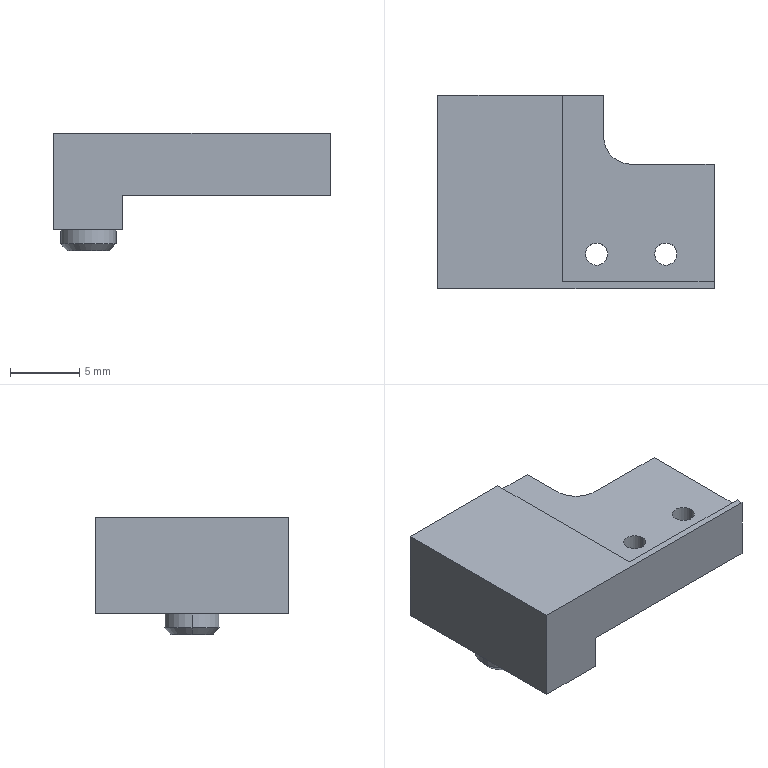Part | STEP file | FBDS-CS-025 | 1 solid | 23 faces | box 20 x 14 x 8.5 mm | volume 1206 mm3 | plane 14 | cylinder 7 | cone 2 | commonest cylinder face diameters 1.6 x4 4 x3
STEP:
#1=CARTESIAN_POINT('',(0.9663,-7.,-4.));
#2=VERTEX_POINT('',#1);
#3=CARTESIAN_POINT('',(4.034,-7.,-4.));
#4=VERTEX_POINT('',#3);
#5=CARTESIAN_POINT('',(2.5,-7.,-4.));
#6=DIRECTION('',(0.,0.,-1.));
#7=DIRECTION('',(-1.,0.,0.));
#8=AXIS2_PLACEMENT_3D('',#5,#6,#7);
#9=CIRCLE('',#8,1.534);
#10=EDGE_CURVE('',#2,#4,#9,.T.);
#11=ORIENTED_EDGE('',*,*,#10,.F.);
#12=CARTESIAN_POINT('',(0.5,-7.,-3.5));
#13=VERTEX_POINT('',#12);
#14=CARTESIAN_POINT('',(0.9663,-7.,-4.));
#15=DIRECTION('',(-0.682,0.,0.7314));
#16=VECTOR('',#15,1000.);
#17=LINE('',#14,#16);
#18=EDGE_CURVE('',#2,#13,#17,.T.);
#19=ORIENTED_EDGE('',*,*,#18,.T.);
#20=CARTESIAN_POINT('',(4.5,-7.,-3.5));
#21=VERTEX_POINT('',#20);
#22=CARTESIAN_POINT('',(2.5,-7.,-3.5));
#23=DIRECTION('',(0.,0.,1.));
#24=DIRECTION('',(-1.,0.,0.));
#25=AXIS2_PLACEMENT_3D('',#22,#23,#24);
#26=CIRCLE('',#25,2.);
#27=EDGE_CURVE('',#21,#13,#26,.T.);
#28=ORIENTED_EDGE('',*,*,#27,.F.);
#29=CARTESIAN_POINT('',(4.034,-7.,-4.));
#30=DIRECTION('',(0.682,0.,0.7314));
#31=VECTOR('',#30,1000.);
#32=LINE('',#29,#31);
#33=EDGE_CURVE('',#4,#21,#32,.T.);
#34=ORIENTED_EDGE('',*,*,#33,.F.);
#35=EDGE_LOOP('',(#11,#19,#28,#34));
#36=FACE_OUTER_BOUND('',#35,.T.);
#37=CARTESIAN_POINT('',(2.5,-7.,-4.));
#38=DIRECTION('',(0.,0.,1.));
#39=DIRECTION('',(1.,0.,0.));
#40=AXIS2_PLACEMENT_3D('',#37,#38,#39);
#41=CONICAL_SURFACE('',#40,1.534,0.7505);
#42=ADVANCED_FACE('',(#36),#41,.T.);
#43=ORIENTED_EDGE('',*,*,#27,.T.);
#44=CARTESIAN_POINT('',(0.5,-7.,-2.5));
#45=VERTEX_POINT('',#44);
#46=CARTESIAN_POINT('',(0.5,-7.,-4.));
#47=DIRECTION('',(0.,0.,1.));
#48=VECTOR('',#47,1000.);
#49=LINE('',#46,#48);
#50=EDGE_CURVE('',#13,#45,#49,.T.);
#51=ORIENTED_EDGE('',*,*,#50,.T.);
#52=CARTESIAN_POINT('',(4.5,-7.,-2.5));
#53=VERTEX_POINT('',#52);
#54=CARTESIAN_POINT('',(2.5,-7.,-2.5));
#55=DIRECTION('',(0.,0.,-1.));
#56=DIRECTION('',(-1.,0.,0.));
#57=AXIS2_PLACEMENT_3D('',#54,#55,#56);
#58=CIRCLE('',#57,2.);
#59=EDGE_CURVE('',#45,#53,#58,.T.);
#60=ORIENTED_EDGE('',*,*,#59,.T.);
#61=CARTESIAN_POINT('',(4.5,-7.,-4.));
#62=DIRECTION('',(0.,0.,1.));
#63=VECTOR('',#62,1000.);
#64=LINE('',#61,#63);
#65=EDGE_CURVE('',#21,#53,#64,.T.);
#66=ORIENTED_EDGE('',*,*,#65,.F.);
#67=EDGE_LOOP('',(#43,#51,#60,#66));
#68=FACE_OUTER_BOUND('',#67,.T.);
#69=CARTESIAN_POINT('',(2.5,-7.,-4.));
#70=DIRECTION('',(0.,0.,1.));
#71=DIRECTION('',(1.,0.,0.));
#72=AXIS2_PLACEMENT_3D('',#69,#70,#71);
#73=CYLINDRICAL_SURFACE('',#72,2.);
#74=ADVANCED_FACE('',(#68),#73,.T.);
#75=CARTESIAN_POINT('',(10.7,-11.5,0.));
#76=VERTEX_POINT('',#75);
#77=CARTESIAN_POINT('',(12.3,-11.5,0.));
#78=VERTEX_POINT('',#77);
#79=CARTESIAN_POINT('',(11.5,-11.5,0.));
#80=DIRECTION('',(0.,0.,1.));
#81=DIRECTION('',(1.,0.,0.));
#82=AXIS2_PLACEMENT_3D('',#79,#80,#81);
#83=CIRCLE('',#82,0.8);
#84=EDGE_CURVE('',#76,#78,#83,.T.);
#85=ORIENTED_EDGE('',*,*,#84,.F.);
#86=CARTESIAN_POINT('',(10.7,-11.5,4.));
#87=VERTEX_POINT('',#86);
#88=CARTESIAN_POINT('',(10.7,-11.5,4.));
#89=DIRECTION('',(0.,0.,1.));
#90=VECTOR('',#89,1000.);
#91=LINE('',#88,#90);
#92=EDGE_CURVE('',#76,#87,#91,.T.);
#93=ORIENTED_EDGE('',*,*,#92,.T.);
#94=CARTESIAN_POINT('',(12.3,-11.5,4.));
#95=VERTEX_POINT('',#94);
#96=CARTESIAN_POINT('',(11.5,-11.5,4.));
#97=DIRECTION('',(0.,0.,1.));
#98=DIRECTION('',(1.,0.,0.));
#99=AXIS2_PLACEMENT_3D('',#96,#97,#98);
#100=CIRCLE('',#99,0.8);
#101=EDGE_CURVE('',#87,#95,#100,.T.);
#102=ORIENTED_EDGE('',*,*,#101,.T.);
#103=CARTESIAN_POINT('',(12.3,-11.5,4.));
#104=DIRECTION('',(0.,0.,1.));
#105=VECTOR('',#104,1000.);
#106=LINE('',#103,#105);
#107=EDGE_CURVE('',#78,#95,#106,.T.);
#108=ORIENTED_EDGE('',*,*,#107,.F.);
#109=EDGE_LOOP('',(#85,#93,#102,#108));
#110=FACE_OUTER_BOUND('',#109,.T.);
#111=CARTESIAN_POINT('',(11.5,-11.5,4.));
#112=DIRECTION('',(0.,0.,1.));
#113=DIRECTION('',(1.,0.,0.));
#114=AXIS2_PLACEMENT_3D('',#111,#112,#113);
#115=CYLINDRICAL_SURFACE('',#114,0.8);
#116=ADVANCED_FACE('',(#110),#115,.F.);
#117=CARTESIAN_POINT('',(15.7,-11.5,0.));
#118=VERTEX_POINT('',#117);
#119=CARTESIAN_POINT('',(17.3,-11.5,0.));
#120=VERTEX_POINT('',#119);
#121=CARTESIAN_POINT('',(16.5,-11.5,0.));
#122=DIRECTION('',(0.,0.,1.));
#123=DIRECTION('',(1.,0.,0.));
#124=AXIS2_PLACEMENT_3D('',#121,#122,#123);
#125=CIRCLE('',#124,0.8);
#126=EDGE_CURVE('',#118,#120,#125,.T.);
#127=ORIENTED_EDGE('',*,*,#126,.F.);
#128=CARTESIAN_POINT('',(15.7,-11.5,4.));
#129=VERTEX_POINT('',#128);
#130=CARTESIAN_POINT('',(15.7,-11.5,4.));
#131=DIRECTION('',(0.,0.,1.));
#132=VECTOR('',#131,1000.);
#133=LINE('',#130,#132);
#134=EDGE_CURVE('',#118,#129,#133,.T.);
#135=ORIENTED_EDGE('',*,*,#134,.T.);
#136=CARTESIAN_POINT('',(17.3,-11.5,4.));
#137=VERTEX_POINT('',#136);
#138=CARTESIAN_POINT('',(16.5,-11.5,4.));
#139=DIRECTION('',(0.,0.,1.));
#140=DIRECTION('',(1.,0.,0.));
#141=AXIS2_PLACEMENT_3D('',#138,#139,#140);
#142=CIRCLE('',#141,0.8);
#143=EDGE_CURVE('',#129,#137,#142,.T.);
#144=ORIENTED_EDGE('',*,*,#143,.T.);
#145=CARTESIAN_POINT('',(17.3,-11.5,4.));
#146=DIRECTION('',(0.,0.,1.));
#147=VECTOR('',#146,1000.);
#148=LINE('',#145,#147);
#149=EDGE_CURVE('',#120,#137,#148,.T.);
#150=ORIENTED_EDGE('',*,*,#149,.F.);
#151=EDGE_LOOP('',(#127,#135,#144,#150));
#152=FACE_OUTER_BOUND('',#151,.T.);
#153=CARTESIAN_POINT('',(16.5,-11.5,4.));
#154=DIRECTION('',(0.,0.,1.));
#155=DIRECTION('',(1.,0.,0.));
#156=AXIS2_PLACEMENT_3D('',#153,#154,#155);
#157=CYLINDRICAL_SURFACE('',#156,0.8);
#158=ADVANCED_FACE('',(#152),#157,.F.);
#159=CARTESIAN_POINT('',(16.5,-11.5,0.));
#160=DIRECTION('',(0.,0.,1.));
#161=DIRECTION('',(1.,0.,0.));
#162=AXIS2_PLACEMENT_3D('',#159,#160,#161);
#163=CIRCLE('',#162,0.8);
#164=EDGE_CURVE('',#120,#118,#163,.T.);
#165=ORIENTED_EDGE('',*,*,#164,.T.);
#166=ORIENTED_EDGE('',*,*,#126,.T.);
#167=EDGE_LOOP('',(#165,#166));
#168=FACE_BOUND('',#167,.T.);
#169=CARTESIAN_POINT('',(11.5,-11.5,0.));
#170=DIRECTION('',(0.,0.,1.));
#171=DIRECTION('',(1.,0.,0.));
#172=AXIS2_PLACEMENT_3D('',#169,#170,#171);
#173=CIRCLE('',#172,0.8);
#174=EDGE_CURVE('',#78,#76,#173,.T.);
#175=ORIENTED_EDGE('',*,*,#174,.T.);
#176=ORIENTED_EDGE('',*,*,#84,.T.);
#177=EDGE_LOOP('',(#175,#176));
#178=FACE_BOUND('',#177,.T.);
#179=CARTESIAN_POINT('',(5.,-14.,0.));
#180=VERTEX_POINT('',#179);
#181=CARTESIAN_POINT('',(20.,-14.,0.));
#182=VERTEX_POINT('',#181);
#183=CARTESIAN_POINT('',(0.,-14.,0.));
#184=DIRECTION('',(1.,0.,0.));
#185=VECTOR('',#184,1000.);
#186=LINE('',#183,#185);
#187=EDGE_CURVE('',#180,#182,#186,.T.);
#188=ORIENTED_EDGE('',*,*,#187,.F.);
#189=CARTESIAN_POINT('',(5.,0.,0.));
#190=VERTEX_POINT('',#189);
#191=CARTESIAN_POINT('',(5.,0.,0.));
#192=DIRECTION('',(0.,1.,0.));
#193=VECTOR('',#192,1000.);
#194=LINE('',#191,#193);
#195=EDGE_CURVE('',#180,#190,#194,.T.);
#196=ORIENTED_EDGE('',*,*,#195,.T.);
#197=CARTESIAN_POINT('',(12.,0.,0.));
#198=VERTEX_POINT('',#197);
#199=CARTESIAN_POINT('',(0.,0.,0.));
#200=DIRECTION('',(-1.,0.,0.));
#201=VECTOR('',#200,1000.);
#202=LINE('',#199,#201);
#203=EDGE_CURVE('',#198,#190,#202,.T.);
#204=ORIENTED_EDGE('',*,*,#203,.F.);
#205=CARTESIAN_POINT('',(12.,-3.,0.));
#206=VERTEX_POINT('',#205);
#207=CARTESIAN_POINT('',(12.,0.,0.));
#208=DIRECTION('',(0.,-1.,0.));
#209=VECTOR('',#208,1000.);
#210=LINE('',#207,#209);
#211=EDGE_CURVE('',#198,#206,#210,.T.);
#212=ORIENTED_EDGE('',*,*,#211,.T.);
#213=CARTESIAN_POINT('',(14.,-5.,0.));
#214=VERTEX_POINT('',#213);
#215=CARTESIAN_POINT('',(14.,-3.,0.));
#216=DIRECTION('',(0.,0.,1.));
#217=DIRECTION('',(1.,0.,0.));
#218=AXIS2_PLACEMENT_3D('',#215,#216,#217);
#219=CIRCLE('',#218,2.);
#220=EDGE_CURVE('',#206,#214,#219,.T.);
#221=ORIENTED_EDGE('',*,*,#220,.T.);
#222=CARTESIAN_POINT('',(20.,-5.,0.));
#223=VERTEX_POINT('',#222);
#224=CARTESIAN_POINT('',(0.,-5.,0.));
#225=DIRECTION('',(1.,0.,0.));
#226=VECTOR('',#225,1000.);
#227=LINE('',#224,#226);
#228=EDGE_CURVE('',#214,#223,#227,.T.);
#229=ORIENTED_EDGE('',*,*,#228,.T.);
#230=CARTESIAN_POINT('',(20.,0.,0.));
#231=DIRECTION('',(0.,1.,0.));
#232=VECTOR('',#231,1000.);
#233=LINE('',#230,#232);
#234=EDGE_CURVE('',#182,#223,#233,.T.);
#235=ORIENTED_EDGE('',*,*,#234,.F.);
#236=EDGE_LOOP('',(#188,#196,#204,#212,#221,#229,#235));
#237=FACE_OUTER_BOUND('',#236,.T.);
#238=CARTESIAN_POINT('',(0.,0.,0.));
#239=DIRECTION('',(0.,0.,1.));
#240=DIRECTION('',(1.,0.,0.));
#241=AXIS2_PLACEMENT_3D('',#238,#239,#240);
#242=PLANE('',#241);
#243=ADVANCED_FACE('',(#168,#178,#237),#242,.F.);
#244=CARTESIAN_POINT('',(20.,-13.5,4.5));
#245=VERTEX_POINT('',#244);
#246=CARTESIAN_POINT('',(20.,-13.5,4.));
#247=VERTEX_POINT('',#246);
#248=CARTESIAN_POINT('',(20.,-13.5,4.5));
#249=DIRECTION('',(0.,0.,-1.));
#250=VECTOR('',#249,1000.);
#251=LINE('',#248,#250);
#252=EDGE_CURVE('',#245,#247,#251,.T.);
#253=ORIENTED_EDGE('',*,*,#252,.F.);
#254=CARTESIAN_POINT('',(20.,-14.,4.5));
#255=VERTEX_POINT('',#254);
#256=CARTESIAN_POINT('',(20.,0.,4.5));
#257=DIRECTION('',(0.,1.,0.));
#258=VECTOR('',#257,1000.);
#259=LINE('',#256,#258);
#260=EDGE_CURVE('',#255,#245,#259,.T.);
#261=ORIENTED_EDGE('',*,*,#260,.F.);
#262=CARTESIAN_POINT('',(20.,-14.,4.5));
#263=DIRECTION('',(0.,0.,-1.));
#264=VECTOR('',#263,1000.);
#265=LINE('',#262,#264);
#266=EDGE_CURVE('',#255,#182,#265,.T.);
#267=ORIENTED_EDGE('',*,*,#266,.T.);
#268=ORIENTED_EDGE('',*,*,#234,.T.);
#269=CARTESIAN_POINT('',(20.,-5.,4.));
#270=VERTEX_POINT('',#269);
#271=CARTESIAN_POINT('',(20.,-5.,-5.5));
#272=DIRECTION('',(0.,0.,1.));
#273=VECTOR('',#272,1000.);
#274=LINE('',#271,#273);
#275=EDGE_CURVE('',#223,#270,#274,.T.);
#276=ORIENTED_EDGE('',*,*,#275,.T.);
#277=CARTESIAN_POINT('',(20.,0.,4.));
#278=DIRECTION('',(0.,-1.,0.));
#279=VECTOR('',#278,1000.);
#280=LINE('',#277,#279);
#281=EDGE_CURVE('',#270,#247,#280,.T.);
#282=ORIENTED_EDGE('',*,*,#281,.T.);
#283=EDGE_LOOP('',(#253,#261,#267,#268,#276,#282));
#284=FACE_OUTER_BOUND('',#283,.T.);
#285=CARTESIAN_POINT('',(20.,0.,4.5));
#286=DIRECTION('',(-1.,0.,0.));
#287=DIRECTION('',(0.,0.,1.));
#288=AXIS2_PLACEMENT_3D('',#285,#286,#287);
#289=PLANE('',#288);
#290=ADVANCED_FACE('',(#284),#289,.F.);
#291=CARTESIAN_POINT('',(9.,0.,4.));
#292=VERTEX_POINT('',#291);
#293=CARTESIAN_POINT('',(9.,0.,4.5));
#294=VERTEX_POINT('',#293);
#295=CARTESIAN_POINT('',(9.,0.,4.5));
#296=DIRECTION('',(0.,0.,1.));
#297=VECTOR('',#296,1000.);
#298=LINE('',#295,#297);
#299=EDGE_CURVE('',#292,#294,#298,.T.);
#300=ORIENTED_EDGE('',*,*,#299,.F.);
#301=CARTESIAN_POINT('',(12.,0.,4.));
#302=VERTEX_POINT('',#301);
#303=CARTESIAN_POINT('',(0.,0.,4.));
#304=DIRECTION('',(1.,0.,0.));
#305=VECTOR('',#304,1000.);
#306=LINE('',#303,#305);
#307=EDGE_CURVE('',#292,#302,#306,.T.);
#308=ORIENTED_EDGE('',*,*,#307,.T.);
#309=CARTESIAN_POINT('',(12.,0.,-5.5));
#310=DIRECTION('',(0.,0.,1.));
#311=VECTOR('',#310,1000.);
#312=LINE('',#309,#311);
#313=EDGE_CURVE('',#198,#302,#312,.T.);
#314=ORIENTED_EDGE('',*,*,#313,.F.);
#315=ORIENTED_EDGE('',*,*,#203,.T.);
#316=CARTESIAN_POINT('',(5.,0.,-2.5));
#317=VERTEX_POINT('',#316);
#318=CARTESIAN_POINT('',(5.,0.,-2.5));
#319=DIRECTION('',(0.,0.,1.));
#320=VECTOR('',#319,1000.);
#321=LINE('',#318,#320);
#322=EDGE_CURVE('',#317,#190,#321,.T.);
#323=ORIENTED_EDGE('',*,*,#322,.F.);
#324=CARTESIAN_POINT('',(0.,0.,-2.5));
#325=VERTEX_POINT('',#324);
#326=CARTESIAN_POINT('',(0.,0.,-2.5));
#327=DIRECTION('',(-1.,0.,0.));
#328=VECTOR('',#327,1000.);
#329=LINE('',#326,#328);
#330=EDGE_CURVE('',#317,#325,#329,.T.);
#331=ORIENTED_EDGE('',*,*,#330,.T.);
#332=CARTESIAN_POINT('',(0.,0.,4.5));
#333=VERTEX_POINT('',#332);
#334=CARTESIAN_POINT('',(0.,0.,4.5));
#335=DIRECTION('',(0.,0.,-1.));
#336=VECTOR('',#335,1000.);
#337=LINE('',#334,#336);
#338=EDGE_CURVE('',#333,#325,#337,.T.);
#339=ORIENTED_EDGE('',*,*,#338,.F.);
#340=CARTESIAN_POINT('',(0.,0.,4.5));
#341=DIRECTION('',(-1.,0.,0.));
#342=VECTOR('',#341,1000.);
#343=LINE('',#340,#342);
#344=EDGE_CURVE('',#294,#333,#343,.T.);
#345=ORIENTED_EDGE('',*,*,#344,.F.);
#346=EDGE_LOOP('',(#300,#308,#314,#315,#323,#331,#339,#345));
#347=FACE_OUTER_BOUND('',#346,.T.);
#348=CARTESIAN_POINT('',(0.,0.,4.5));
#349=DIRECTION('',(0.,-1.,0.));
#350=DIRECTION('',(0.,0.,-1.));
#351=AXIS2_PLACEMENT_3D('',#348,#349,#350);
#352=PLANE('',#351);
#353=ADVANCED_FACE('',(#347),#352,.F.);
#354=CARTESIAN_POINT('',(9.,-13.5,4.5));
#355=VERTEX_POINT('',#354);
#356=CARTESIAN_POINT('',(28.367,-13.5,4.5));
#357=DIRECTION('',(-1.,0.,0.));
#358=VECTOR('',#357,1000.);
#359=LINE('',#356,#358);
#360=EDGE_CURVE('',#245,#355,#359,.T.);
#361=ORIENTED_EDGE('',*,*,#360,.T.);
#362=CARTESIAN_POINT('',(9.,1.393,4.5));
#363=DIRECTION('',(0.,1.,0.));
#364=VECTOR('',#363,1000.);
#365=LINE('',#362,#364);
#366=EDGE_CURVE('',#355,#294,#365,.T.);
#367=ORIENTED_EDGE('',*,*,#366,.T.);
#368=ORIENTED_EDGE('',*,*,#344,.T.);
#369=CARTESIAN_POINT('',(0.,-14.,4.5));
#370=VERTEX_POINT('',#369);
#371=CARTESIAN_POINT('',(0.,0.,4.5));
#372=DIRECTION('',(0.,-1.,0.));
#373=VECTOR('',#372,1000.);
#374=LINE('',#371,#373);
#375=EDGE_CURVE('',#333,#370,#374,.T.);
#376=ORIENTED_EDGE('',*,*,#375,.T.);
#377=CARTESIAN_POINT('',(0.,-14.,4.5));
#378=DIRECTION('',(1.,0.,0.));
#379=VECTOR('',#378,1000.);
#380=LINE('',#377,#379);
#381=EDGE_CURVE('',#370,#255,#380,.T.);
#382=ORIENTED_EDGE('',*,*,#381,.T.);
#383=ORIENTED_EDGE('',*,*,#260,.T.);
#384=EDGE_LOOP('',(#361,#367,#368,#376,#382,#383));
#385=FACE_OUTER_BOUND('',#384,.T.);
#386=CARTESIAN_POINT('',(0.,0.,4.5));
#387=DIRECTION('',(0.,0.,1.));
#388=DIRECTION('',(1.,0.,0.));
#389=AXIS2_PLACEMENT_3D('',#386,#387,#388);
#390=PLANE('',#389);
#391=ADVANCED_FACE('',(#385),#390,.T.);
#392=ORIENTED_EDGE('',*,*,#338,.T.);
#393=CARTESIAN_POINT('',(0.,-14.,-2.5));
#394=VERTEX_POINT('',#393);
#395=CARTESIAN_POINT('',(0.,0.,-2.5));
#396=DIRECTION('',(0.,-1.,0.));
#397=VECTOR('',#396,1000.);
#398=LINE('',#395,#397);
#399=EDGE_CURVE('',#325,#394,#398,.T.);
#400=ORIENTED_EDGE('',*,*,#399,.T.);
#401=CARTESIAN_POINT('',(0.,-14.,14.5));
#402=DIRECTION('',(0.,0.,-1.));
#403=VECTOR('',#402,1000.);
#404=LINE('',#401,#403);
#405=EDGE_CURVE('',#370,#394,#404,.T.);
#406=ORIENTED_EDGE('',*,*,#405,.F.);
#407=ORIENTED_EDGE('',*,*,#375,.F.);
#408=EDGE_LOOP('',(#392,#400,#406,#407));
#409=FACE_OUTER_BOUND('',#408,.T.);
#410=CARTESIAN_POINT('',(0.,0.,4.5));
#411=DIRECTION('',(1.,0.,0.));
#412=DIRECTION('',(0.,1.,0.));
#413=AXIS2_PLACEMENT_3D('',#410,#411,#412);
#414=PLANE('',#413);
#415=ADVANCED_FACE('',(#409),#414,.F.);
#416=ORIENTED_EDGE('',*,*,#381,.F.);
#417=ORIENTED_EDGE('',*,*,#405,.T.);
#418=CARTESIAN_POINT('',(5.,-14.,-2.5));
#419=VERTEX_POINT('',#418);
#420=CARTESIAN_POINT('',(5.,-14.,-2.5));
#421=DIRECTION('',(1.,0.,0.));
#422=VECTOR('',#421,1000.);
#423=LINE('',#420,#422);
#424=EDGE_CURVE('',#394,#419,#423,.T.);
#425=ORIENTED_EDGE('',*,*,#424,.T.);
#426=CARTESIAN_POINT('',(5.,-14.,-10.31));
#427=DIRECTION('',(0.,0.,1.));
#428=VECTOR('',#427,1000.);
#429=LINE('',#426,#428);
#430=EDGE_CURVE('',#419,#180,#429,.T.);
#431=ORIENTED_EDGE('',*,*,#430,.T.);
#432=ORIENTED_EDGE('',*,*,#187,.T.);
#433=ORIENTED_EDGE('',*,*,#266,.F.);
#434=EDGE_LOOP('',(#416,#417,#425,#431,#432,#433));
#435=FACE_OUTER_BOUND('',#434,.T.);
#436=CARTESIAN_POINT('',(0.,-14.,4.5));
#437=DIRECTION('',(0.,1.,0.));
#438=DIRECTION('',(0.,0.,1.));
#439=AXIS2_PLACEMENT_3D('',#436,#437,#438);
#440=PLANE('',#439);
#441=ADVANCED_FACE('',(#435),#440,.F.);
#442=ORIENTED_EDGE('',*,*,#228,.F.);
#443=CARTESIAN_POINT('',(14.,-5.,4.));
#444=VERTEX_POINT('',#443);
#445=CARTESIAN_POINT('',(14.,-5.,4.));
#446=DIRECTION('',(0.,0.,1.));
#447=VECTOR('',#446,1000.);
#448=LINE('',#445,#447);
#449=EDGE_CURVE('',#214,#444,#448,.T.);
#450=ORIENTED_EDGE('',*,*,#449,.T.);
#451=CARTESIAN_POINT('',(20.,-5.,4.));
#452=DIRECTION('',(1.,0.,0.));
#453=VECTOR('',#452,1000.);
#454=LINE('',#451,#453);
#455=EDGE_CURVE('',#444,#270,#454,.T.);
#456=ORIENTED_EDGE('',*,*,#455,.T.);
#457=ORIENTED_EDGE('',*,*,#275,.F.);
#458=EDGE_LOOP('',(#442,#450,#456,#457));
#459=FACE_OUTER_BOUND('',#458,.T.);
#460=CARTESIAN_POINT('',(20.,-5.,-5.5));
#461=DIRECTION('',(0.,-1.,0.));
#462=DIRECTION('',(1.,0.,0.));
#463=AXIS2_PLACEMENT_3D('',#460,#461,#462);
#464=PLANE('',#463);
#465=ADVANCED_FACE('',(#459),#464,.F.);
#466=CARTESIAN_POINT('',(12.,-3.,4.));
#467=VERTEX_POINT('',#466);
#468=CARTESIAN_POINT('',(12.,0.,4.));
#469=DIRECTION('',(0.,-1.,0.));
#470=VECTOR('',#469,1000.);
#471=LINE('',#468,#470);
#472=EDGE_CURVE('',#302,#467,#471,.T.);
#473=ORIENTED_EDGE('',*,*,#472,.T.);
#474=CARTESIAN_POINT('',(12.,-3.,0.));
#475=DIRECTION('',(0.,0.,-1.));
#476=VECTOR('',#475,1000.);
#477=LINE('',#474,#476);
#478=EDGE_CURVE('',#467,#206,#477,.T.);
#479=ORIENTED_EDGE('',*,*,#478,.T.);
#480=ORIENTED_EDGE('',*,*,#211,.F.);
#481=ORIENTED_EDGE('',*,*,#313,.T.);
#482=EDGE_LOOP('',(#473,#479,#480,#481));
#483=FACE_OUTER_BOUND('',#482,.T.);
#484=CARTESIAN_POINT('',(12.,0.,-5.5));
#485=DIRECTION('',(-1.,0.,0.));
#486=DIRECTION('',(0.,0.,1.));
#487=AXIS2_PLACEMENT_3D('',#484,#485,#486);
#488=PLANE('',#487);
#489=ADVANCED_FACE('',(#483),#488,.F.);
#490=CARTESIAN_POINT('',(9.,-13.5,4.));
#491=VERTEX_POINT('',#490);
#492=CARTESIAN_POINT('',(9.,-13.5,0.8377));
#493=DIRECTION('',(0.,0.,1.));
#494=VECTOR('',#493,1000.);
#495=LINE('',#492,#494);
#496=EDGE_CURVE('',#491,#355,#495,.T.);
#497=ORIENTED_EDGE('',*,*,#496,.T.);
#498=ORIENTED_EDGE('',*,*,#360,.F.);
#499=ORIENTED_EDGE('',*,*,#252,.T.);
#500=CARTESIAN_POINT('',(28.367,-13.5,4.));
#501=DIRECTION('',(-1.,0.,0.));
#502=VECTOR('',#501,1000.);
#503=LINE('',#500,#502);
#504=EDGE_CURVE('',#247,#491,#503,.T.);
#505=ORIENTED_EDGE('',*,*,#504,.T.);
#506=EDGE_LOOP('',(#497,#498,#499,#505));
#507=FACE_OUTER_BOUND('',#506,.T.);
#508=CARTESIAN_POINT('',(28.367,-13.5,4.));
#509=DIRECTION('',(0.,1.,0.));
#510=DIRECTION('',(0.,0.,1.));
#511=AXIS2_PLACEMENT_3D('',#508,#509,#510);
#512=PLANE('',#511);
#513=ADVANCED_FACE('',(#507),#512,.T.);
#514=ORIENTED_EDGE('',*,*,#366,.F.);
#515=ORIENTED_EDGE('',*,*,#496,.F.);
#516=CARTESIAN_POINT('',(9.,1.393,4.));
#517=DIRECTION('',(0.,1.,0.));
#518=VECTOR('',#517,1000.);
#519=LINE('',#516,#518);
#520=EDGE_CURVE('',#491,#292,#519,.T.);
#521=ORIENTED_EDGE('',*,*,#520,.T.);
#522=ORIENTED_EDGE('',*,*,#299,.T.);
#523=EDGE_LOOP('',(#514,#515,#521,#522));
#524=FACE_OUTER_BOUND('',#523,.T.);
#525=CARTESIAN_POINT('',(9.,1.393,4.));
#526=DIRECTION('',(1.,0.,0.));
#527=DIRECTION('',(0.,1.,0.));
#528=AXIS2_PLACEMENT_3D('',#525,#526,#527);
#529=PLANE('',#528);
#530=ADVANCED_FACE('',(#524),#529,.T.);
#531=CARTESIAN_POINT('',(11.5,-11.5,4.));
#532=DIRECTION('',(0.,0.,1.));
#533=DIRECTION('',(1.,0.,0.));
#534=AXIS2_PLACEMENT_3D('',#531,#532,#533);
#535=CIRCLE('',#534,0.8);
#536=EDGE_CURVE('',#95,#87,#535,.T.);
#537=ORIENTED_EDGE('',*,*,#536,.F.);
#538=ORIENTED_EDGE('',*,*,#101,.F.);
#539=EDGE_LOOP('',(#537,#538));
#540=FACE_BOUND('',#539,.T.);
#541=CARTESIAN_POINT('',(16.5,-11.5,4.));
#542=DIRECTION('',(0.,0.,1.));
#543=DIRECTION('',(1.,0.,0.));
#544=AXIS2_PLACEMENT_3D('',#541,#542,#543);
#545=CIRCLE('',#544,0.8);
#546=EDGE_CURVE('',#137,#129,#545,.T.);
#547=ORIENTED_EDGE('',*,*,#546,.F.);
#548=ORIENTED_EDGE('',*,*,#143,.F.);
#549=EDGE_LOOP('',(#547,#548));
#550=FACE_BOUND('',#549,.T.);
#551=ORIENTED_EDGE('',*,*,#520,.F.);
#552=ORIENTED_EDGE('',*,*,#504,.F.);
#553=ORIENTED_EDGE('',*,*,#281,.F.);
#554=ORIENTED_EDGE('',*,*,#455,.F.);
#555=CARTESIAN_POINT('',(14.,-3.,4.));
#556=DIRECTION('',(0.,0.,-1.));
#557=DIRECTION('',(-1.,0.,0.));
#558=AXIS2_PLACEMENT_3D('',#555,#556,#557);
#559=CIRCLE('',#558,2.);
#560=EDGE_CURVE('',#444,#467,#559,.T.);
#561=ORIENTED_EDGE('',*,*,#560,.T.);
#562=ORIENTED_EDGE('',*,*,#472,.F.);
#563=ORIENTED_EDGE('',*,*,#307,.F.);
#564=EDGE_LOOP('',(#551,#552,#553,#554,#561,#562,#563));
#565=FACE_OUTER_BOUND('',#564,.T.);
#566=CARTESIAN_POINT('',(0.,0.,4.));
#567=DIRECTION('',(0.,0.,-1.));
#568=DIRECTION('',(-1.,0.,0.));
#569=AXIS2_PLACEMENT_3D('',#566,#567,#568);
#570=PLANE('',#569);
#571=ADVANCED_FACE('',(#540,#550,#565),#570,.F.);
#572=ORIENTED_EDGE('',*,*,#134,.F.);
#573=ORIENTED_EDGE('',*,*,#164,.F.);
#574=ORIENTED_EDGE('',*,*,#149,.T.);
#575=ORIENTED_EDGE('',*,*,#546,.T.);
#576=EDGE_LOOP('',(#572,#573,#574,#575));
#577=FACE_OUTER_BOUND('',#576,.T.);
#578=CARTESIAN_POINT('',(16.5,-11.5,4.));
#579=DIRECTION('',(0.,0.,1.));
#580=DIRECTION('',(1.,0.,0.));
#581=AXIS2_PLACEMENT_3D('',#578,#579,#580);
#582=CYLINDRICAL_SURFACE('',#581,0.8);
#583=ADVANCED_FACE('',(#577),#582,.F.);
#584=ORIENTED_EDGE('',*,*,#92,.F.);
#585=ORIENTED_EDGE('',*,*,#174,.F.);
#586=ORIENTED_EDGE('',*,*,#107,.T.);
#587=ORIENTED_EDGE('',*,*,#536,.T.);
#588=EDGE_LOOP('',(#584,#585,#586,#587));
#589=FACE_OUTER_BOUND('',#588,.T.);
#590=CARTESIAN_POINT('',(11.5,-11.5,4.));
#591=DIRECTION('',(0.,0.,1.));
#592=DIRECTION('',(1.,0.,0.));
#593=AXIS2_PLACEMENT_3D('',#590,#591,#592);
#594=CYLINDRICAL_SURFACE('',#593,0.8);
#595=ADVANCED_FACE('',(#589),#594,.F.);
#596=ORIENTED_EDGE('',*,*,#220,.F.);
#597=ORIENTED_EDGE('',*,*,#478,.F.);
#598=ORIENTED_EDGE('',*,*,#560,.F.);
#599=ORIENTED_EDGE('',*,*,#449,.F.);
#600=EDGE_LOOP('',(#596,#597,#598,#599));
#601=FACE_OUTER_BOUND('',#600,.T.);
#602=CARTESIAN_POINT('',(14.,-3.,-5.5));
#603=DIRECTION('',(0.,0.,-1.));
#604=DIRECTION('',(-1.,0.,0.));
#605=AXIS2_PLACEMENT_3D('',#602,#603,#604);
#606=CYLINDRICAL_SURFACE('',#605,2.);
#607=ADVANCED_FACE('',(#601),#606,.F.);
#608=ORIENTED_EDGE('',*,*,#195,.F.);
#609=ORIENTED_EDGE('',*,*,#430,.F.);
#610=CARTESIAN_POINT('',(5.,0.,-2.5));
#611=DIRECTION('',(0.,1.,0.));
#612=VECTOR('',#611,1000.);
#613=LINE('',#610,#612);
#614=EDGE_CURVE('',#419,#317,#613,.T.);
#615=ORIENTED_EDGE('',*,*,#614,.T.);
#616=ORIENTED_EDGE('',*,*,#322,.T.);
#617=EDGE_LOOP('',(#608,#609,#615,#616));
#618=FACE_OUTER_BOUND('',#617,.T.);
#619=CARTESIAN_POINT('',(5.,0.,-2.5));
#620=DIRECTION('',(1.,0.,0.));
#621=DIRECTION('',(0.,1.,0.));
#622=AXIS2_PLACEMENT_3D('',#619,#620,#621);
#623=PLANE('',#622);
#624=ADVANCED_FACE('',(#618),#623,.T.);
#625=CARTESIAN_POINT('',(2.5,-7.,-2.5));
#626=DIRECTION('',(0.,0.,-1.));
#627=DIRECTION('',(-1.,0.,0.));
#628=AXIS2_PLACEMENT_3D('',#625,#626,#627);
#629=CIRCLE('',#628,2.);
#630=EDGE_CURVE('',#53,#45,#629,.T.);
#631=ORIENTED_EDGE('',*,*,#630,.F.);
#632=ORIENTED_EDGE('',*,*,#59,.F.);
#633=EDGE_LOOP('',(#631,#632));
#634=FACE_BOUND('',#633,.T.);
#635=ORIENTED_EDGE('',*,*,#399,.F.);
#636=ORIENTED_EDGE('',*,*,#330,.F.);
#637=ORIENTED_EDGE('',*,*,#614,.F.);
#638=ORIENTED_EDGE('',*,*,#424,.F.);
#639=EDGE_LOOP('',(#635,#636,#637,#638));
#640=FACE_OUTER_BOUND('',#639,.T.);
#641=CARTESIAN_POINT('',(0.,0.,-2.5));
#642=DIRECTION('',(0.,0.,1.));
#643=DIRECTION('',(1.,0.,0.));
#644=AXIS2_PLACEMENT_3D('',#641,#642,#643);
#645=PLANE('',#644);
#646=ADVANCED_FACE('',(#634,#640),#645,.F.);
#647=ORIENTED_EDGE('',*,*,#50,.F.);
#648=CARTESIAN_POINT('',(2.5,-7.,-3.5));
#649=DIRECTION('',(0.,0.,1.));
#650=DIRECTION('',(-1.,0.,0.));
#651=AXIS2_PLACEMENT_3D('',#648,#649,#650);
#652=CIRCLE('',#651,2.);
#653=EDGE_CURVE('',#13,#21,#652,.T.);
#654=ORIENTED_EDGE('',*,*,#653,.T.);
#655=ORIENTED_EDGE('',*,*,#65,.T.);
#656=ORIENTED_EDGE('',*,*,#630,.T.);
#657=EDGE_LOOP('',(#647,#654,#655,#656));
#658=FACE_OUTER_BOUND('',#657,.T.);
#659=CARTESIAN_POINT('',(2.5,-7.,-4.));
#660=DIRECTION('',(0.,0.,1.));
#661=DIRECTION('',(1.,0.,0.));
#662=AXIS2_PLACEMENT_3D('',#659,#660,#661);
#663=CYLINDRICAL_SURFACE('',#662,2.);
#664=ADVANCED_FACE('',(#658),#663,.T.);
#665=CARTESIAN_POINT('',(2.5,-7.,-4.));
#666=DIRECTION('',(0.,0.,-1.));
#667=DIRECTION('',(-1.,0.,0.));
#668=AXIS2_PLACEMENT_3D('',#665,#666,#667);
#669=CIRCLE('',#668,1.534);
#670=EDGE_CURVE('',#4,#2,#669,.T.);
#671=ORIENTED_EDGE('',*,*,#670,.T.);
#672=ORIENTED_EDGE('',*,*,#10,.T.);
#673=EDGE_LOOP('',(#671,#672));
#674=FACE_OUTER_BOUND('',#673,.T.);
#675=CARTESIAN_POINT('',(2.5,-7.,-4.));
#676=DIRECTION('',(0.,0.,-1.));
#677=DIRECTION('',(-1.,0.,0.));
#678=AXIS2_PLACEMENT_3D('',#675,#676,#677);
#679=PLANE('',#678);
#680=ADVANCED_FACE('',(#674),#679,.T.);
#681=ORIENTED_EDGE('',*,*,#18,.F.);
#682=ORIENTED_EDGE('',*,*,#670,.F.);
#683=ORIENTED_EDGE('',*,*,#33,.T.);
#684=ORIENTED_EDGE('',*,*,#653,.F.);
#685=EDGE_LOOP('',(#681,#682,#683,#684));
#686=FACE_OUTER_BOUND('',#685,.T.);
#687=CARTESIAN_POINT('',(2.5,-7.,-4.));
#688=DIRECTION('',(0.,0.,1.));
#689=DIRECTION('',(1.,0.,0.));
#690=AXIS2_PLACEMENT_3D('',#687,#688,#689);
#691=CONICAL_SURFACE('',#690,1.534,0.7505);
#692=ADVANCED_FACE('',(#686),#691,.T.);
#693=CLOSED_SHELL('',(#42,#74,#116,#158,#243,#290,#353,#391,#415,#441,#465,#489,#513,#530,#571,#583,#595,#607,#624,#646,#664,#680,#692));
#694=MANIFOLD_SOLID_BREP('',#693);
#695=CARTESIAN_POINT('',(0.,0.,0.));
#696=DIRECTION('',(0.,0.,1.));
#697=DIRECTION('',(1.,0.,0.));
#698=AXIS2_PLACEMENT_3D('',#695,#696,#697);
#699=(LENGTH_UNIT()NAMED_UNIT(*)SI_UNIT(.MILLI.,.METRE.));
#700=UNCERTAINTY_MEASURE_WITH_UNIT(LENGTH_MEASURE(0.00001),#699,'','');
#701=(NAMED_UNIT(*)PLANE_ANGLE_UNIT()SI_UNIT($,.RADIAN.));
#702=(NAMED_UNIT(*)SI_UNIT($,.STERADIAN.)SOLID_ANGLE_UNIT());
#703=(GEOMETRIC_REPRESENTATION_CONTEXT(3)GLOBAL_UNCERTAINTY_ASSIGNED_CONTEXT((#700))GLOBAL_UNIT_ASSIGNED_CONTEXT((#699,#701,#702))REPRESENTATION_CONTEXT('',''));
#704=ADVANCED_BREP_SHAPE_REPRESENTATION('',(#694,#698),#703);